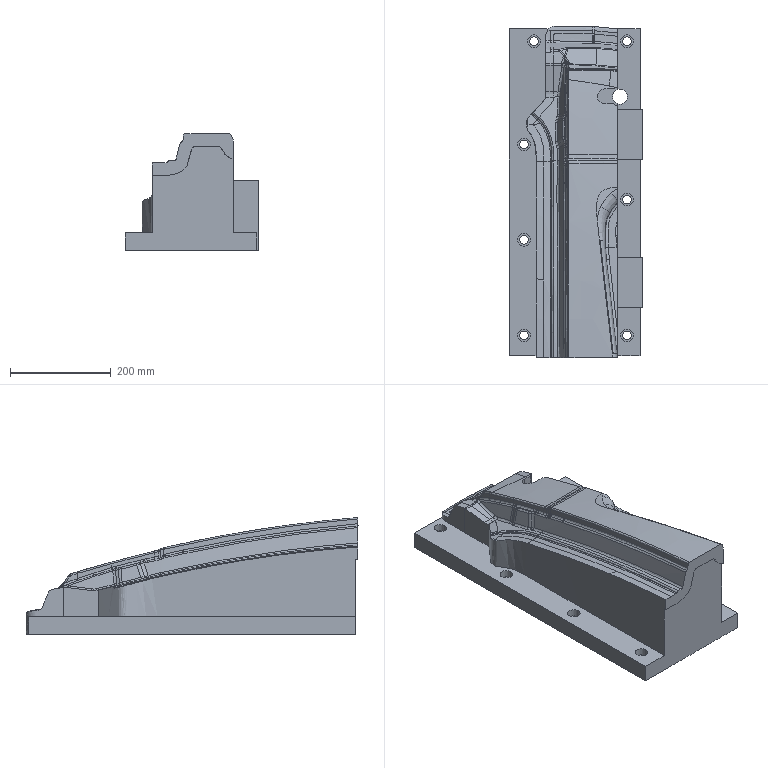Part | NX | features solid 2 | 1 solid | 289 faces | box 265 x 660.516 x 232.404 mm | volume 14784849 mm3 | spline 175 | cylinder 64 | plane 46 | sphere 4 | commonest cylinder face diameters 17 x7 25 x7 40 x4 10.002 x3 6.004 x2 9.99 x2